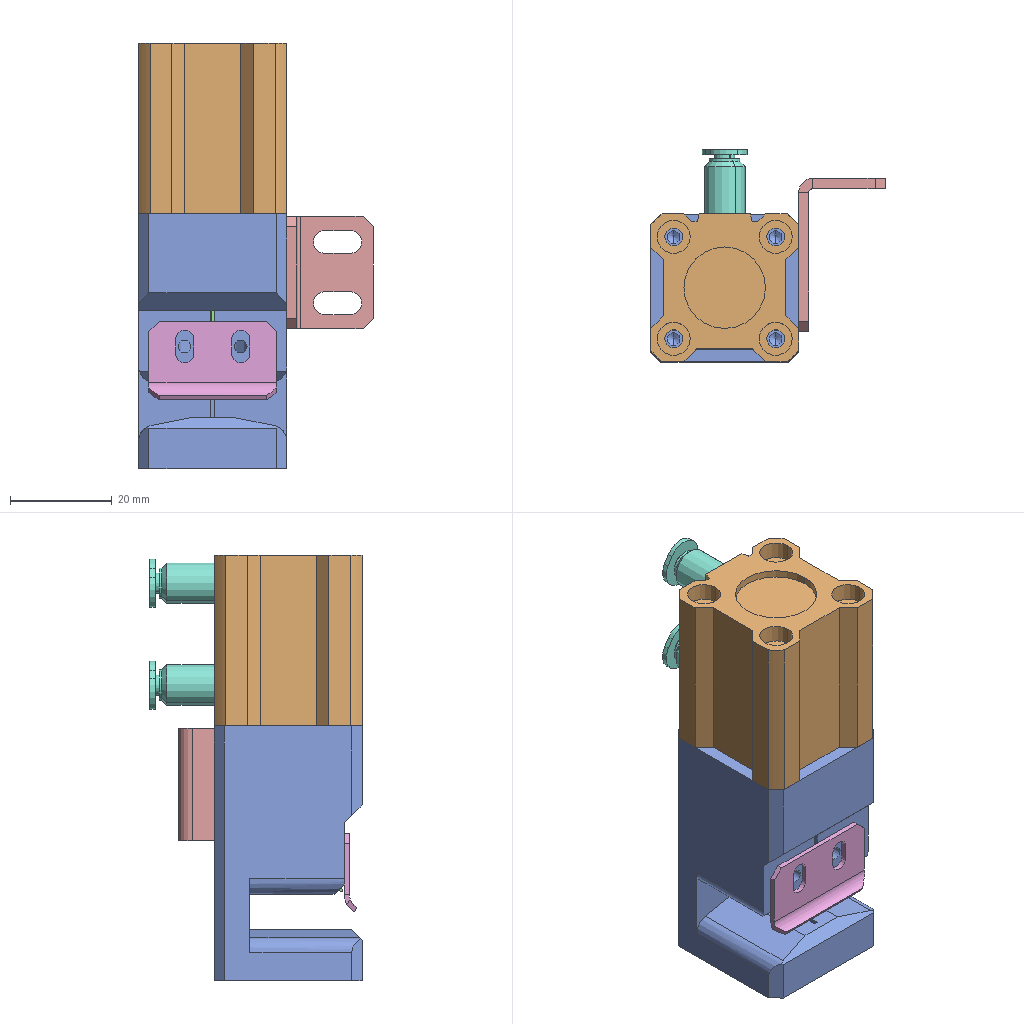Assembly | SolidWorks | 10 different items | 14 placed | box 46 x 42 x 84 mm
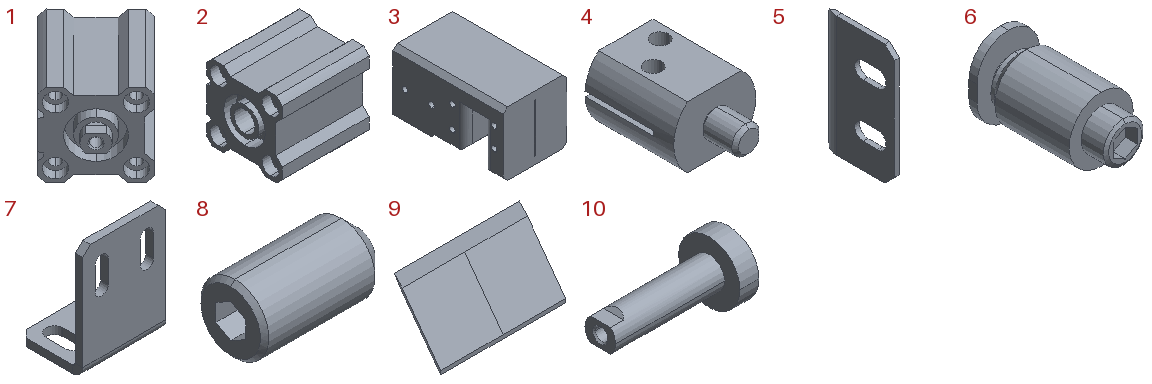Parts list (item | name | quantity | parent item | size | volume | features):
1 | (subassembly) | x1 | - | 44.194 x 44.194 x 29 mm | 19135 mm3 | -
2 | - | x1 | in 1 | 33.5 x 29 x 29 mm | 16795 mm3 | features RefAxis 3, HoleWzd 2, LPattern 2, RevCut 2, 3DProfileFeature 1, Extrusion 1, ICE 1
3 | - | x1 | - | 29 x 50 x 29 mm | 27875 mm3 | features HoleWzd 5, ICE 5, Chamfer 4, Fillet 2, Extrusion 1
4 | - | x1 | - | 12 x 18 x 9 mm | 1174 mm3 | features ICE 5, Chamfer 1, Extrusion 1, HoleWzd 1, RevCut 1
5 | - | x1 | - | 2.5 x 15.464 x 25 mm | 343.263 mm3 | features Chamfer 1, FlatPattern 1, Hem 1, ICE 1, SMBaseFlange 1, SheetMetal 1
6 | - | x2 | - | 8 x 15.6 x 9.8 mm | 520.13 mm3 | features BaseBody 1
7 | - | x1 | - | 22 x 17 x 30 mm | 1655 mm3 | features ICE 2, Chamfer 1, EdgeFlange 1, FlatPattern 1, SMBaseFlange 1, SheetMetal 1
8 | - | x4 | - | 3 x 1.6 x 1.6 mm | 5.35 mm3 | features RevCut 2, Cut 1, LPattern 1, Revolution 1
9 | - | x1 | - | 30.104 x 17.5 x 0.6 mm | 192 mm3 | features PLine 2, Extrusion 1, ICE 1, MirrorPattern 1
10 | - | x1 | in 1 | 33.5 x 16 x 16 mm | 2340 mm3 | features RefAxis 3, 3DProfileFeature 1, ICE 1, Revolution 1
Mates (type | each side: item.copy, entity, surface, feature):
In the top assembly
Concentric | 10.1 face cylinder Revolve1 | 4.1 face cylinder Cut-Extrude1
Coincident | 10.1 face plane Revolve1 | 4.1 face plane Cut-Extrude1
Coincident | 4.1 face plane Cut-Extrude2 | 9.1 face plane Split Line2
Coincident | 4.1 face plane Cut-Extrude2 | 9.1 face plane Boss-Extrude1
DistanceDim | 4.1 edge | 9.1 edge
Concentric | 4.1 face cylinder M3 Tapped Hole1 | 8.1 face cylinder Base
Concentric | 4.1 face cylinder M3 Tapped Hole1 | 8.2 face cylinder Base
Concentric | 4.1 face cylinder M3 Tapped Hole1 | 8.3 face cylinder Base
Concentric | 4.1 face cylinder M3 Tapped Hole1 | 8.4 face cylinder Base
Coincident | 9.1 face plane Split Line1 | 8.1 face plane Base
Coincident | 9.1 face plane Split Line1 | 8.2 face plane Base
Coincident | 9.1 face plane Split Line2 | 8.3 edge
Coincident | 9.1 face plane Split Line2 | 8.4 face plane Base
Concentric | 10.1 face cylinder Revolve1 | 3.1 face cylinder Cut-Extrude8
Parallel | 4.1 face plane Cut-Extrude3 | 3.1 face plane Boss-Extrude1
Concentric | 2.1 face cylinder LPattern2 | 3.1 face cylinder M3 Tapped Hole1
Coincident | 2.1 face plane Boss-Extrude1 | 3.1 face plane Boss-Extrude1
Coincident | 5.1 face plane Base-Flange1 | 3.1 face plane Cut-Extrude7
DistanceDim | 5.1 face plane Base-Flange1 | 3.1 face plane Boss-Extrude1
Coincident | 3.1 face plane Cut-Extrude7 | 5.1 face plane Base-Flange1
Coincident | 3.1 face plane Boss-Extrude1 | 7.1 face plane Base-Flange1
DistanceDim | 7.1 face plane Base-Flange1 | 3.1 face plane Boss-Extrude1
DistanceDim | 3.1 face plane Boss-Extrude1 | 7.1 face plane Base-Flange1
Concentric | 6.1 face cylinder Input1 | 2.1 face cylinder Hole2
Concentric | 6.2 face cylinder Input1 | 2.1 face cylinder LPattern1
Coincident | 6.1 face plane Input1 | 2.1 face plane Boss-Extrude1
Coincident | 6.2 face plane Input1 | 2.1 face plane Boss-Extrude1
In subassembly 1
Coincident | 2.2 axis | 10.2 axis
PlanarAngleDim | 10.2 plane | 2.2 plane
LimitDistanceDim | 10.2 face plane Revolve1 | 2.2 face plane Boss-Extrude1